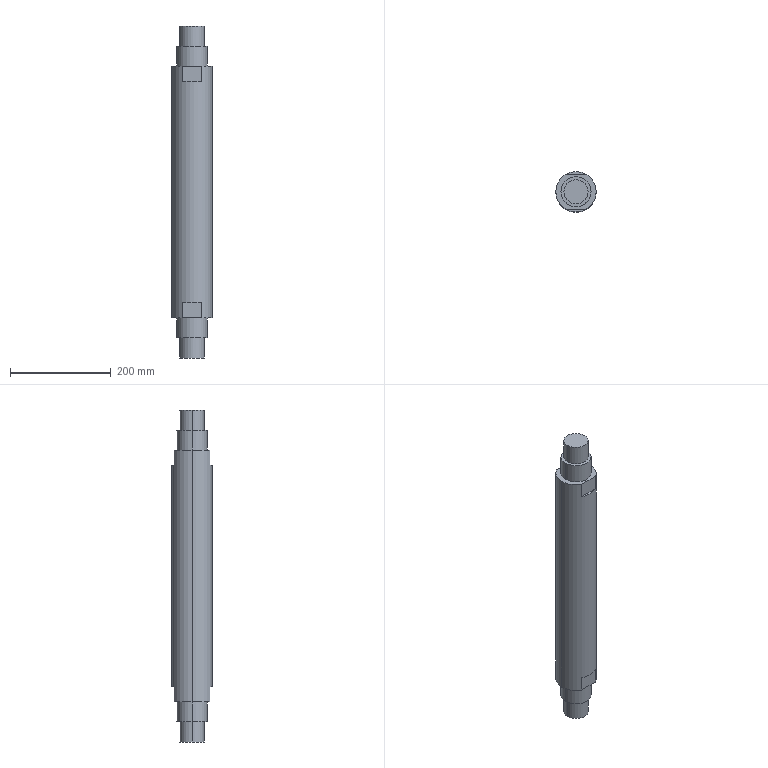Part | STEP file | 001-009-Riveting guide pin | 1 solid | 24 faces | box 80 x 80 x 659 mm | volume 2865709 mm3 | plane 14 | cylinder 10 | commonest cylinder face diameters 48 x4 60 x4 80 x2